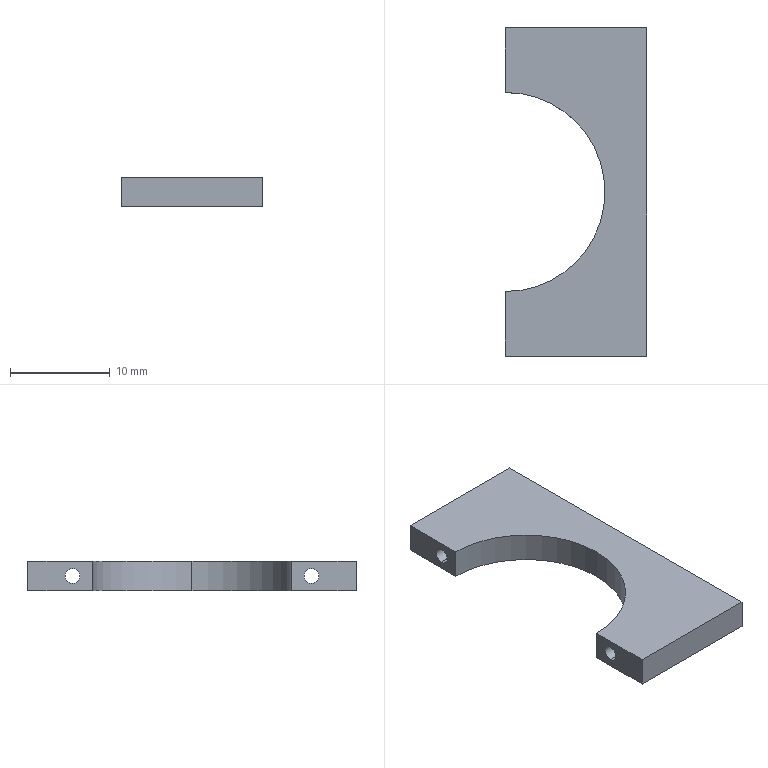Part | SolidWorks | features Cut 1, Extrusion 1 | 1 solid | 13 faces | box 14.182 x 33 x 3 mm | volume 882.699 mm3 | plane 7 | cylinder 6 | commonest cylinder face diameters 1.5 x4 20 x2
STEP:
#1=CARTESIAN_POINT('',(16.5,1.996,-0.75));
#2=VERTEX_POINT('',#1);
#3=CARTESIAN_POINT('',(16.5,1.996,-2.25));
#4=VERTEX_POINT('',#3);
#5=CARTESIAN_POINT('',(16.5,1.996,-1.5));
#6=DIRECTION('',(1.,0.,0.));
#7=DIRECTION('',(0.,0.,1.));
#8=AXIS2_PLACEMENT_3D('',#5,#6,#7);
#9=CIRCLE('',#8,0.75);
#10=EDGE_CURVE('',#2,#4,#9,.T.);
#11=ORIENTED_EDGE('',*,*,#10,.F.);
#12=CARTESIAN_POINT('',(30.682,1.996,-0.75));
#13=VERTEX_POINT('',#12);
#14=CARTESIAN_POINT('',(16.5,1.996,-0.75));
#15=DIRECTION('',(1.,0.,0.));
#16=VECTOR('',#15,1000.);
#17=LINE('',#14,#16);
#18=EDGE_CURVE('',#2,#13,#17,.T.);
#19=ORIENTED_EDGE('',*,*,#18,.T.);
#20=CARTESIAN_POINT('',(30.682,1.996,-2.25));
#21=VERTEX_POINT('',#20);
#22=CARTESIAN_POINT('',(30.682,1.996,-1.5));
#23=DIRECTION('',(1.,0.,0.));
#24=DIRECTION('',(0.,0.,1.));
#25=AXIS2_PLACEMENT_3D('',#22,#23,#24);
#26=CIRCLE('',#25,0.75);
#27=EDGE_CURVE('',#13,#21,#26,.T.);
#28=ORIENTED_EDGE('',*,*,#27,.T.);
#29=CARTESIAN_POINT('',(16.5,1.996,-2.25));
#30=DIRECTION('',(1.,0.,0.));
#31=VECTOR('',#30,1000.);
#32=LINE('',#29,#31);
#33=EDGE_CURVE('',#4,#21,#32,.T.);
#34=ORIENTED_EDGE('',*,*,#33,.F.);
#35=EDGE_LOOP('',(#11,#19,#28,#34));
#36=FACE_OUTER_BOUND('',#35,.T.);
#37=CARTESIAN_POINT('',(16.5,1.996,-1.5));
#38=DIRECTION('',(1.,0.,0.));
#39=DIRECTION('',(0.,0.,-1.));
#40=AXIS2_PLACEMENT_3D('',#37,#38,#39);
#41=CYLINDRICAL_SURFACE('',#40,0.75);
#42=ADVANCED_FACE('',(#36),#41,.F.);
#43=CARTESIAN_POINT('',(16.5,-22.004,-0.75));
#44=VERTEX_POINT('',#43);
#45=CARTESIAN_POINT('',(16.5,-22.004,-2.25));
#46=VERTEX_POINT('',#45);
#47=CARTESIAN_POINT('',(16.5,-22.004,-1.5));
#48=DIRECTION('',(1.,0.,0.));
#49=DIRECTION('',(0.,0.,-1.));
#50=AXIS2_PLACEMENT_3D('',#47,#48,#49);
#51=CIRCLE('',#50,0.75);
#52=EDGE_CURVE('',#44,#46,#51,.T.);
#53=ORIENTED_EDGE('',*,*,#52,.F.);
#54=CARTESIAN_POINT('',(30.682,-22.004,-0.75));
#55=VERTEX_POINT('',#54);
#56=CARTESIAN_POINT('',(16.5,-22.004,-0.75));
#57=DIRECTION('',(1.,0.,0.));
#58=VECTOR('',#57,1000.);
#59=LINE('',#56,#58);
#60=EDGE_CURVE('',#44,#55,#59,.T.);
#61=ORIENTED_EDGE('',*,*,#60,.T.);
#62=CARTESIAN_POINT('',(30.682,-22.004,-2.25));
#63=VERTEX_POINT('',#62);
#64=CARTESIAN_POINT('',(30.682,-22.004,-1.5));
#65=DIRECTION('',(1.,0.,0.));
#66=DIRECTION('',(0.,0.,-1.));
#67=AXIS2_PLACEMENT_3D('',#64,#65,#66);
#68=CIRCLE('',#67,0.75);
#69=EDGE_CURVE('',#55,#63,#68,.T.);
#70=ORIENTED_EDGE('',*,*,#69,.T.);
#71=CARTESIAN_POINT('',(16.5,-22.004,-2.25));
#72=DIRECTION('',(1.,0.,0.));
#73=VECTOR('',#72,1000.);
#74=LINE('',#71,#73);
#75=EDGE_CURVE('',#46,#63,#74,.T.);
#76=ORIENTED_EDGE('',*,*,#75,.F.);
#77=EDGE_LOOP('',(#53,#61,#70,#76));
#78=FACE_OUTER_BOUND('',#77,.T.);
#79=CARTESIAN_POINT('',(16.5,-22.004,-1.5));
#80=DIRECTION('',(1.,0.,0.));
#81=DIRECTION('',(0.,0.,-1.));
#82=AXIS2_PLACEMENT_3D('',#79,#80,#81);
#83=CYLINDRICAL_SURFACE('',#82,0.75);
#84=ADVANCED_FACE('',(#78),#83,.F.);
#85=CARTESIAN_POINT('',(16.5,-0.004132,-3.));
#86=VERTEX_POINT('',#85);
#87=CARTESIAN_POINT('',(26.5,-10.004,-3.));
#88=VERTEX_POINT('',#87);
#89=CARTESIAN_POINT('',(16.5,-10.004,-3.));
#90=DIRECTION('',(0.,0.,-1.));
#91=DIRECTION('',(1.,0.,0.));
#92=AXIS2_PLACEMENT_3D('',#89,#90,#91);
#93=CIRCLE('',#92,10.);
#94=EDGE_CURVE('',#86,#88,#93,.T.);
#95=ORIENTED_EDGE('',*,*,#94,.T.);
#96=CARTESIAN_POINT('',(26.5,-10.004,0.));
#97=VERTEX_POINT('',#96);
#98=CARTESIAN_POINT('',(26.5,-10.004,-3.));
#99=DIRECTION('',(0.,0.,1.));
#100=VECTOR('',#99,1000.);
#101=LINE('',#98,#100);
#102=EDGE_CURVE('',#88,#97,#101,.T.);
#103=ORIENTED_EDGE('',*,*,#102,.T.);
#104=CARTESIAN_POINT('',(16.5,-0.004132,0.));
#105=VERTEX_POINT('',#104);
#106=CARTESIAN_POINT('',(16.5,-10.004,0.));
#107=DIRECTION('',(0.,0.,-1.));
#108=DIRECTION('',(1.,0.,0.));
#109=AXIS2_PLACEMENT_3D('',#106,#107,#108);
#110=CIRCLE('',#109,10.);
#111=EDGE_CURVE('',#105,#97,#110,.T.);
#112=ORIENTED_EDGE('',*,*,#111,.F.);
#113=CARTESIAN_POINT('',(16.5,-0.004132,-3.));
#114=DIRECTION('',(0.,0.,1.));
#115=VECTOR('',#114,1000.);
#116=LINE('',#113,#115);
#117=EDGE_CURVE('',#86,#105,#116,.T.);
#118=ORIENTED_EDGE('',*,*,#117,.F.);
#119=EDGE_LOOP('',(#95,#103,#112,#118));
#120=FACE_OUTER_BOUND('',#119,.T.);
#121=CARTESIAN_POINT('',(16.5,-10.004,-3.));
#122=DIRECTION('',(0.,0.,1.));
#123=DIRECTION('',(1.,0.,0.));
#124=AXIS2_PLACEMENT_3D('',#121,#122,#123);
#125=CYLINDRICAL_SURFACE('',#124,10.);
#126=ADVANCED_FACE('',(#120),#125,.F.);
#127=CARTESIAN_POINT('',(16.5,-22.004,-1.5));
#128=DIRECTION('',(1.,0.,0.));
#129=DIRECTION('',(0.,0.,-1.));
#130=AXIS2_PLACEMENT_3D('',#127,#128,#129);
#131=CIRCLE('',#130,0.75);
#132=EDGE_CURVE('',#46,#44,#131,.T.);
#133=ORIENTED_EDGE('',*,*,#132,.T.);
#134=ORIENTED_EDGE('',*,*,#52,.T.);
#135=EDGE_LOOP('',(#133,#134));
#136=FACE_BOUND('',#135,.T.);
#137=CARTESIAN_POINT('',(16.5,-20.004,0.));
#138=VERTEX_POINT('',#137);
#139=CARTESIAN_POINT('',(16.5,-26.504,0.));
#140=VERTEX_POINT('',#139);
#141=CARTESIAN_POINT('',(16.5,-26.504,0.));
#142=DIRECTION('',(0.,-1.,0.));
#143=VECTOR('',#142,1000.);
#144=LINE('',#141,#143);
#145=EDGE_CURVE('',#138,#140,#144,.T.);
#146=ORIENTED_EDGE('',*,*,#145,.F.);
#147=CARTESIAN_POINT('',(16.5,-20.004,-3.));
#148=VERTEX_POINT('',#147);
#149=CARTESIAN_POINT('',(16.5,-20.004,-3.));
#150=DIRECTION('',(0.,0.,1.));
#151=VECTOR('',#150,1000.);
#152=LINE('',#149,#151);
#153=EDGE_CURVE('',#148,#138,#152,.T.);
#154=ORIENTED_EDGE('',*,*,#153,.F.);
#155=CARTESIAN_POINT('',(16.5,-26.504,-3.));
#156=VERTEX_POINT('',#155);
#157=CARTESIAN_POINT('',(16.5,-26.504,-3.));
#158=DIRECTION('',(0.,-1.,0.));
#159=VECTOR('',#158,1000.);
#160=LINE('',#157,#159);
#161=EDGE_CURVE('',#148,#156,#160,.T.);
#162=ORIENTED_EDGE('',*,*,#161,.T.);
#163=CARTESIAN_POINT('',(16.5,-26.504,-3.));
#164=DIRECTION('',(0.,0.,1.));
#165=VECTOR('',#164,1000.);
#166=LINE('',#163,#165);
#167=EDGE_CURVE('',#156,#140,#166,.T.);
#168=ORIENTED_EDGE('',*,*,#167,.T.);
#169=EDGE_LOOP('',(#146,#154,#162,#168));
#170=FACE_OUTER_BOUND('',#169,.T.);
#171=CARTESIAN_POINT('',(16.5,-26.504,-3.));
#172=DIRECTION('',(-1.,0.,0.));
#173=DIRECTION('',(0.,0.,1.));
#174=AXIS2_PLACEMENT_3D('',#171,#172,#173);
#175=PLANE('',#174);
#176=ADVANCED_FACE('',(#136,#170),#175,.T.);
#177=ORIENTED_EDGE('',*,*,#102,.F.);
#178=CARTESIAN_POINT('',(16.5,-10.004,-3.));
#179=DIRECTION('',(0.,0.,-1.));
#180=DIRECTION('',(1.,0.,0.));
#181=AXIS2_PLACEMENT_3D('',#178,#179,#180);
#182=CIRCLE('',#181,10.);
#183=EDGE_CURVE('',#88,#148,#182,.T.);
#184=ORIENTED_EDGE('',*,*,#183,.T.);
#185=ORIENTED_EDGE('',*,*,#153,.T.);
#186=CARTESIAN_POINT('',(16.5,-10.004,0.));
#187=DIRECTION('',(0.,0.,-1.));
#188=DIRECTION('',(1.,0.,0.));
#189=AXIS2_PLACEMENT_3D('',#186,#187,#188);
#190=CIRCLE('',#189,10.);
#191=EDGE_CURVE('',#97,#138,#190,.T.);
#192=ORIENTED_EDGE('',*,*,#191,.F.);
#193=EDGE_LOOP('',(#177,#184,#185,#192));
#194=FACE_OUTER_BOUND('',#193,.T.);
#195=CARTESIAN_POINT('',(16.5,-10.004,-3.));
#196=DIRECTION('',(0.,0.,1.));
#197=DIRECTION('',(1.,0.,0.));
#198=AXIS2_PLACEMENT_3D('',#195,#196,#197);
#199=CYLINDRICAL_SURFACE('',#198,10.);
#200=ADVANCED_FACE('',(#194),#199,.F.);
#201=CARTESIAN_POINT('',(16.5,1.996,-1.5));
#202=DIRECTION('',(1.,0.,0.));
#203=DIRECTION('',(0.,0.,1.));
#204=AXIS2_PLACEMENT_3D('',#201,#202,#203);
#205=CIRCLE('',#204,0.75);
#206=EDGE_CURVE('',#4,#2,#205,.T.);
#207=ORIENTED_EDGE('',*,*,#206,.T.);
#208=ORIENTED_EDGE('',*,*,#10,.T.);
#209=EDGE_LOOP('',(#207,#208));
#210=FACE_BOUND('',#209,.T.);
#211=CARTESIAN_POINT('',(16.5,6.496,0.));
#212=VERTEX_POINT('',#211);
#213=CARTESIAN_POINT('',(16.5,6.496,0.));
#214=DIRECTION('',(0.,-1.,0.));
#215=VECTOR('',#214,1000.);
#216=LINE('',#213,#215);
#217=EDGE_CURVE('',#212,#105,#216,.T.);
#218=ORIENTED_EDGE('',*,*,#217,.F.);
#219=CARTESIAN_POINT('',(16.5,6.496,-3.));
#220=VERTEX_POINT('',#219);
#221=CARTESIAN_POINT('',(16.5,6.496,-3.));
#222=DIRECTION('',(0.,0.,1.));
#223=VECTOR('',#222,1000.);
#224=LINE('',#221,#223);
#225=EDGE_CURVE('',#220,#212,#224,.T.);
#226=ORIENTED_EDGE('',*,*,#225,.F.);
#227=CARTESIAN_POINT('',(16.5,6.496,-3.));
#228=DIRECTION('',(0.,-1.,0.));
#229=VECTOR('',#228,1000.);
#230=LINE('',#227,#229);
#231=EDGE_CURVE('',#220,#86,#230,.T.);
#232=ORIENTED_EDGE('',*,*,#231,.T.);
#233=ORIENTED_EDGE('',*,*,#117,.T.);
#234=EDGE_LOOP('',(#218,#226,#232,#233));
#235=FACE_OUTER_BOUND('',#234,.T.);
#236=CARTESIAN_POINT('',(16.5,6.496,-3.));
#237=DIRECTION('',(-1.,0.,0.));
#238=DIRECTION('',(0.,0.,1.));
#239=AXIS2_PLACEMENT_3D('',#236,#237,#238);
#240=PLANE('',#239);
#241=ADVANCED_FACE('',(#210,#235),#240,.T.);
#242=CARTESIAN_POINT('',(30.682,6.496,0.));
#243=VERTEX_POINT('',#242);
#244=CARTESIAN_POINT('',(30.682,6.496,0.));
#245=DIRECTION('',(-1.,0.,0.));
#246=VECTOR('',#245,1000.);
#247=LINE('',#244,#246);
#248=EDGE_CURVE('',#243,#212,#247,.T.);
#249=ORIENTED_EDGE('',*,*,#248,.F.);
#250=CARTESIAN_POINT('',(30.682,6.496,-3.));
#251=VERTEX_POINT('',#250);
#252=CARTESIAN_POINT('',(30.682,6.496,-3.));
#253=DIRECTION('',(0.,0.,1.));
#254=VECTOR('',#253,1000.);
#255=LINE('',#252,#254);
#256=EDGE_CURVE('',#251,#243,#255,.T.);
#257=ORIENTED_EDGE('',*,*,#256,.F.);
#258=CARTESIAN_POINT('',(30.682,6.496,-3.));
#259=DIRECTION('',(-1.,0.,0.));
#260=VECTOR('',#259,1000.);
#261=LINE('',#258,#260);
#262=EDGE_CURVE('',#251,#220,#261,.T.);
#263=ORIENTED_EDGE('',*,*,#262,.T.);
#264=ORIENTED_EDGE('',*,*,#225,.T.);
#265=EDGE_LOOP('',(#249,#257,#263,#264));
#266=FACE_OUTER_BOUND('',#265,.T.);
#267=CARTESIAN_POINT('',(30.682,6.496,-3.));
#268=DIRECTION('',(0.,1.,0.));
#269=DIRECTION('',(0.,0.,1.));
#270=AXIS2_PLACEMENT_3D('',#267,#268,#269);
#271=PLANE('',#270);
#272=ADVANCED_FACE('',(#266),#271,.T.);
#273=CARTESIAN_POINT('',(30.682,1.996,-1.5));
#274=DIRECTION('',(1.,0.,0.));
#275=DIRECTION('',(0.,0.,1.));
#276=AXIS2_PLACEMENT_3D('',#273,#274,#275);
#277=CIRCLE('',#276,0.75);
#278=EDGE_CURVE('',#21,#13,#277,.T.);
#279=ORIENTED_EDGE('',*,*,#278,.F.);
#280=ORIENTED_EDGE('',*,*,#27,.F.);
#281=EDGE_LOOP('',(#279,#280));
#282=FACE_BOUND('',#281,.T.);
#283=CARTESIAN_POINT('',(30.682,-22.004,-1.5));
#284=DIRECTION('',(1.,0.,0.));
#285=DIRECTION('',(0.,0.,-1.));
#286=AXIS2_PLACEMENT_3D('',#283,#284,#285);
#287=CIRCLE('',#286,0.75);
#288=EDGE_CURVE('',#63,#55,#287,.T.);
#289=ORIENTED_EDGE('',*,*,#288,.F.);
#290=ORIENTED_EDGE('',*,*,#69,.F.);
#291=EDGE_LOOP('',(#289,#290));
#292=FACE_BOUND('',#291,.T.);
#293=CARTESIAN_POINT('',(30.682,-26.504,0.));
#294=VERTEX_POINT('',#293);
#295=CARTESIAN_POINT('',(30.682,-26.504,0.));
#296=DIRECTION('',(0.,1.,0.));
#297=VECTOR('',#296,1000.);
#298=LINE('',#295,#297);
#299=EDGE_CURVE('',#294,#243,#298,.T.);
#300=ORIENTED_EDGE('',*,*,#299,.F.);
#301=CARTESIAN_POINT('',(30.682,-26.504,-3.));
#302=VERTEX_POINT('',#301);
#303=CARTESIAN_POINT('',(30.682,-26.504,-3.));
#304=DIRECTION('',(0.,0.,1.));
#305=VECTOR('',#304,1000.);
#306=LINE('',#303,#305);
#307=EDGE_CURVE('',#302,#294,#306,.T.);
#308=ORIENTED_EDGE('',*,*,#307,.F.);
#309=CARTESIAN_POINT('',(30.682,-26.504,-3.));
#310=DIRECTION('',(0.,1.,0.));
#311=VECTOR('',#310,1000.);
#312=LINE('',#309,#311);
#313=EDGE_CURVE('',#302,#251,#312,.T.);
#314=ORIENTED_EDGE('',*,*,#313,.T.);
#315=ORIENTED_EDGE('',*,*,#256,.T.);
#316=EDGE_LOOP('',(#300,#308,#314,#315));
#317=FACE_OUTER_BOUND('',#316,.T.);
#318=CARTESIAN_POINT('',(30.682,-26.504,-3.));
#319=DIRECTION('',(1.,0.,0.));
#320=DIRECTION('',(0.,0.,-1.));
#321=AXIS2_PLACEMENT_3D('',#318,#319,#320);
#322=PLANE('',#321);
#323=ADVANCED_FACE('',(#282,#292,#317),#322,.T.);
#324=CARTESIAN_POINT('',(16.5,-26.504,0.));
#325=DIRECTION('',(1.,0.,0.));
#326=VECTOR('',#325,1000.);
#327=LINE('',#324,#326);
#328=EDGE_CURVE('',#140,#294,#327,.T.);
#329=ORIENTED_EDGE('',*,*,#328,.F.);
#330=ORIENTED_EDGE('',*,*,#167,.F.);
#331=CARTESIAN_POINT('',(16.5,-26.504,-3.));
#332=DIRECTION('',(1.,0.,0.));
#333=VECTOR('',#332,1000.);
#334=LINE('',#331,#333);
#335=EDGE_CURVE('',#156,#302,#334,.T.);
#336=ORIENTED_EDGE('',*,*,#335,.T.);
#337=ORIENTED_EDGE('',*,*,#307,.T.);
#338=EDGE_LOOP('',(#329,#330,#336,#337));
#339=FACE_OUTER_BOUND('',#338,.T.);
#340=CARTESIAN_POINT('',(16.5,-26.504,-3.));
#341=DIRECTION('',(0.,-1.,0.));
#342=DIRECTION('',(0.,0.,-1.));
#343=AXIS2_PLACEMENT_3D('',#340,#341,#342);
#344=PLANE('',#343);
#345=ADVANCED_FACE('',(#339),#344,.T.);
#346=ORIENTED_EDGE('',*,*,#161,.F.);
#347=ORIENTED_EDGE('',*,*,#183,.F.);
#348=ORIENTED_EDGE('',*,*,#94,.F.);
#349=ORIENTED_EDGE('',*,*,#231,.F.);
#350=ORIENTED_EDGE('',*,*,#262,.F.);
#351=ORIENTED_EDGE('',*,*,#313,.F.);
#352=ORIENTED_EDGE('',*,*,#335,.F.);
#353=EDGE_LOOP('',(#346,#347,#348,#349,#350,#351,#352));
#354=FACE_OUTER_BOUND('',#353,.T.);
#355=CARTESIAN_POINT('',(16.5,-10.004,-3.));
#356=DIRECTION('',(0.,0.,1.));
#357=DIRECTION('',(1.,0.,0.));
#358=AXIS2_PLACEMENT_3D('',#355,#356,#357);
#359=PLANE('',#358);
#360=ADVANCED_FACE('',(#354),#359,.F.);
#361=ORIENTED_EDGE('',*,*,#145,.T.);
#362=ORIENTED_EDGE('',*,*,#328,.T.);
#363=ORIENTED_EDGE('',*,*,#299,.T.);
#364=ORIENTED_EDGE('',*,*,#248,.T.);
#365=ORIENTED_EDGE('',*,*,#217,.T.);
#366=ORIENTED_EDGE('',*,*,#111,.T.);
#367=ORIENTED_EDGE('',*,*,#191,.T.);
#368=EDGE_LOOP('',(#361,#362,#363,#364,#365,#366,#367));
#369=FACE_OUTER_BOUND('',#368,.T.);
#370=CARTESIAN_POINT('',(16.5,-10.004,0.));
#371=DIRECTION('',(0.,0.,1.));
#372=DIRECTION('',(1.,0.,0.));
#373=AXIS2_PLACEMENT_3D('',#370,#371,#372);
#374=PLANE('',#373);
#375=ADVANCED_FACE('',(#369),#374,.T.);
#376=ORIENTED_EDGE('',*,*,#60,.F.);
#377=ORIENTED_EDGE('',*,*,#132,.F.);
#378=ORIENTED_EDGE('',*,*,#75,.T.);
#379=ORIENTED_EDGE('',*,*,#288,.T.);
#380=EDGE_LOOP('',(#376,#377,#378,#379));
#381=FACE_OUTER_BOUND('',#380,.T.);
#382=CARTESIAN_POINT('',(16.5,-22.004,-1.5));
#383=DIRECTION('',(1.,0.,0.));
#384=DIRECTION('',(0.,0.,-1.));
#385=AXIS2_PLACEMENT_3D('',#382,#383,#384);
#386=CYLINDRICAL_SURFACE('',#385,0.75);
#387=ADVANCED_FACE('',(#381),#386,.F.);
#388=ORIENTED_EDGE('',*,*,#18,.F.);
#389=ORIENTED_EDGE('',*,*,#206,.F.);
#390=ORIENTED_EDGE('',*,*,#33,.T.);
#391=ORIENTED_EDGE('',*,*,#278,.T.);
#392=EDGE_LOOP('',(#388,#389,#390,#391));
#393=FACE_OUTER_BOUND('',#392,.T.);
#394=CARTESIAN_POINT('',(16.5,1.996,-1.5));
#395=DIRECTION('',(1.,0.,0.));
#396=DIRECTION('',(0.,0.,-1.));
#397=AXIS2_PLACEMENT_3D('',#394,#395,#396);
#398=CYLINDRICAL_SURFACE('',#397,0.75);
#399=ADVANCED_FACE('',(#393),#398,.F.);
#400=CLOSED_SHELL('',(#42,#84,#126,#176,#200,#241,#272,#323,#345,#360,#375,#387,#399));
#401=MANIFOLD_SOLID_BREP('',#400);
#402=CARTESIAN_POINT('',(0.,0.,0.));
#403=DIRECTION('',(0.,0.,1.));
#404=DIRECTION('',(1.,0.,0.));
#405=AXIS2_PLACEMENT_3D('',#402,#403,#404);
#406=(LENGTH_UNIT()NAMED_UNIT(*)SI_UNIT(.MILLI.,.METRE.));
#407=UNCERTAINTY_MEASURE_WITH_UNIT(LENGTH_MEASURE(0.00001),#406,'','');
#408=(NAMED_UNIT(*)PLANE_ANGLE_UNIT()SI_UNIT($,.RADIAN.));
#409=(NAMED_UNIT(*)SI_UNIT($,.STERADIAN.)SOLID_ANGLE_UNIT());
#410=(GEOMETRIC_REPRESENTATION_CONTEXT(3)GLOBAL_UNCERTAINTY_ASSIGNED_CONTEXT((#407))GLOBAL_UNIT_ASSIGNED_CONTEXT((#406,#408,#409))REPRESENTATION_CONTEXT('',''));
#411=ADVANCED_BREP_SHAPE_REPRESENTATION('',(#401,#405),#410);